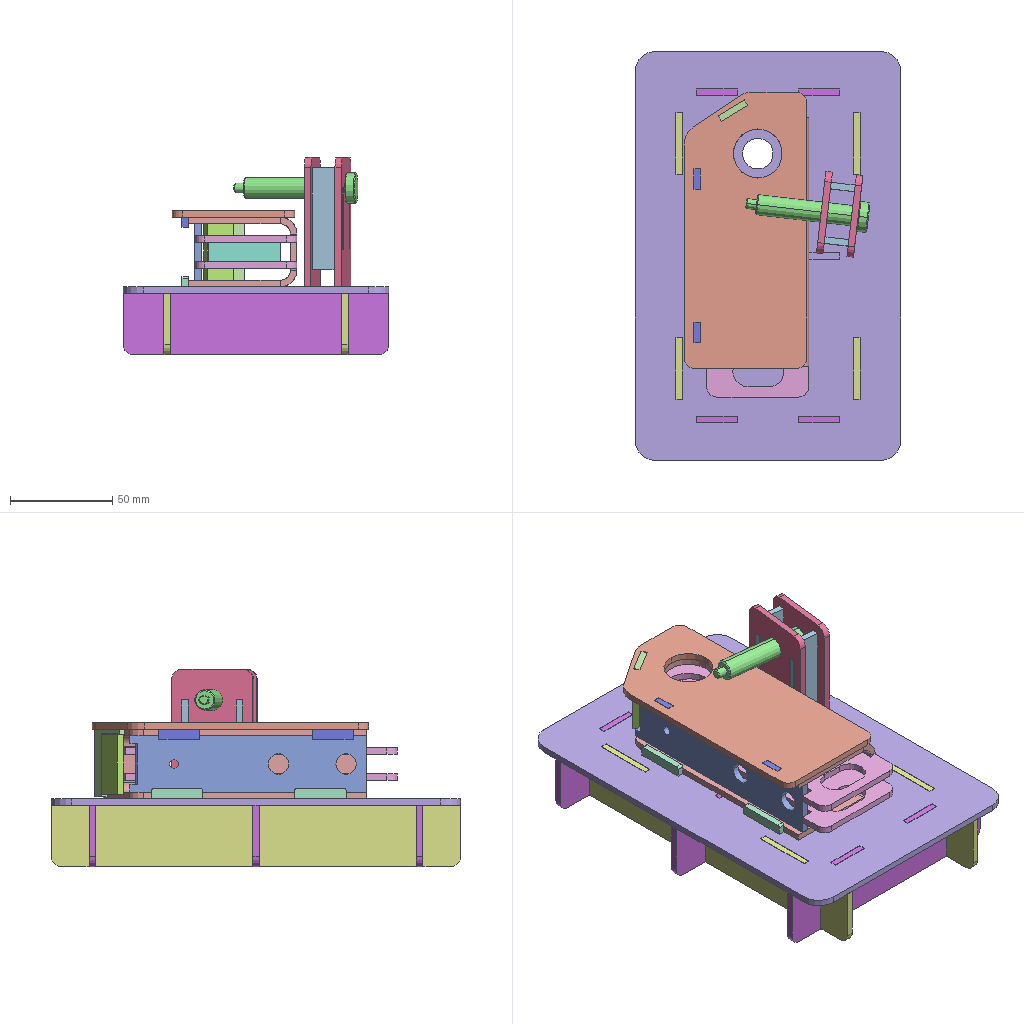Assembly | SolidWorks | 16 different items | 25 placed | box 130 x 200 x 97 mm
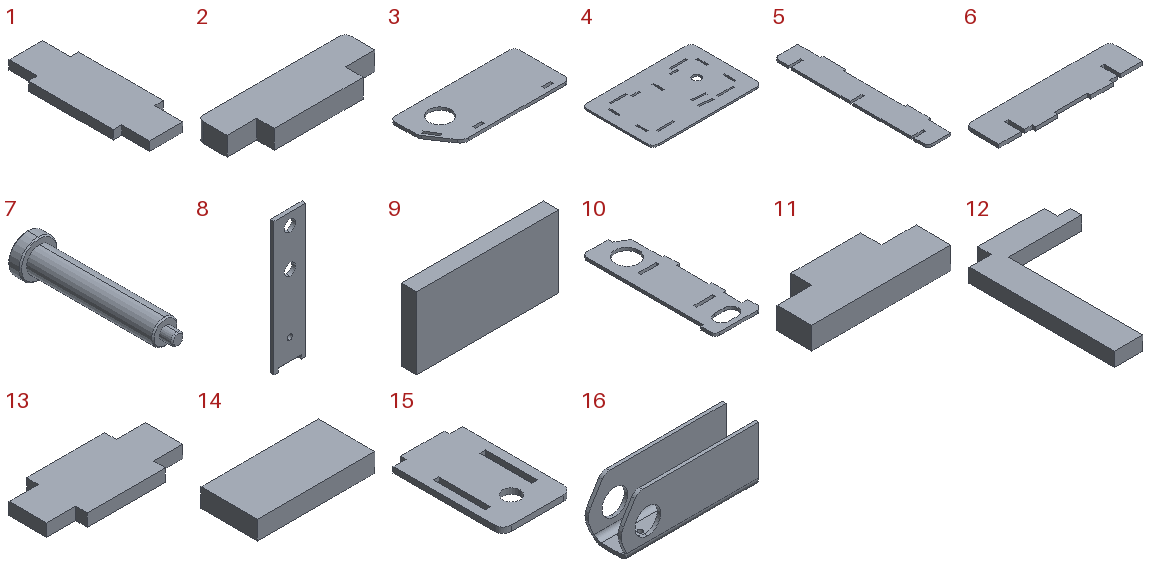Parts list (item | quantity | size | volume | features):
1 | x2 | 17.8 x 50 x 3.2 mm | 2464 mm3 | features FlatPattern 1, SMBaseFlange 1, SheetMetal 1
2 | x2 | 25 x 8 x 3.2 mm | 542.627 mm3 | features FlatPattern 1, SMBaseFlange 1, SheetMetal 1
3 | x1 | 135 x 60 x 3.2 mm | 23086 mm3 | features FlatPattern 1, SMBaseFlange 1, SheetMetal 1
4 | x1 | 200 x 130 x 3.2 mm | 79288 mm3 | features FlatPattern 1, SMBaseFlange 1, SheetMetal 1
5 | x2 | 33 x 200 x 3.2 mm | 19266 mm3 | features FlatPattern 1, SMBaseFlange 1, SheetMetal 1
6 | x3 | 130 x 33 x 3.2 mm | 12522 mm3 | features FlatPattern 1, SMBaseFlange 1, SheetMetal 1
7 | x1 | 15 x 60 x 15 mm | 4886 mm3 | features Chamfer 1, Revolution 1
8 | x1 | 27.6 x 3.2 x 115.6 mm | 9476 mm3 | features Chamfer 1, FlatPattern 1, SMBaseFlange 1, SheetMetal 1
9 | x1 | 29.6 x 3.2 x 15 mm | 1421 mm3 | features FlatPattern 1, SMBaseFlange 1, SheetMetal 1
10 | x2 | 50 x 145 x 3.2 mm | 16071 mm3 | features Fillet 1, FlatPattern 1, SMBaseFlange 1, SheetMetal 1
11 | x2 | 20 x 8 x 3.2 mm | 416 mm3 | features FlatPattern 1, SMBaseFlange 1, SheetMetal 1
12 | x1 | 23 x 36 x 3.2 mm | 953.226 mm3 | features FlatPattern 1, SMBaseFlange 1, SheetMetal 1
13 | x2 | 35 x 15.6 x 3.2 mm | 1459 mm3 | features FlatPattern 1, SMBaseFlange 1, SheetMetal 1
14 | x1 | 20 x 9.6 x 3.2 mm | 614.4 mm3 | features FlatPattern 1, SMBaseFlange 1, SheetMetal 1
15 | x2 | 40 x 66.3 x 3.2 mm | 7442 mm3 | features Fillet 1, FlatPattern 1, SMBaseFlange 1, SheetMetal 1
16 | x1 | 128.757 x 34 x 53 mm | 47449 mm3 | features ICE 2, Fillet 1, FlatPattern 1, SMBaseFlange 1, SheetMetal 1
Mates (type | each side: item.copy, entity, surface, feature):
Coincident | 16.1 face plane Base-Flange1 | 8.1 face plane Base-Flange1 | 2 times
DistanceDim | 16.1 face plane Base-Flange1 | 8.1 face plane Base-Flange1
Coincident | 16.1 face plane Cut-Extrude1 | 9.1 face plane Base-Flange1
DistanceDim | 9.1 face plane Base-Flange1 | 16.1 face plane Base-Flange1
DistanceDim | 9.1 edge | 16.1 face plane Base-Flange1
InPlace | 10.1 plane | assembly plane
InPlace | 13.1 plane | assembly plane
InPlace | 14.1 plane | assembly plane
Coincident | 16.1 face plane Base-Flange1 | 4.1 face plane Base-Flange1
Concentric | 16.1 face cylinder Cut-Extrude1 | 4.1 face cylinder Base-Flange1
Parallel | 16.1 face plane Base-Flange1 | 4.1 face plane Base-Flange1
InPlace | 7.1 face plane Revolve1 | 15.1 plane
InPlace | 1.1 plane | assembly plane
InPlace | 5.1 plane | assembly plane
InPlace | 6.1 plane | assembly plane
InPlace | 16.1 face plane Base-Flange1 | 2.1 plane
InPlace | 16.1 face plane Base-Flange1 | 3.1 plane
InPlace | 16.1 face plane Base-Flange1 | 11.1 plane
InPlace | 16.1 face plane Cut-Extrude1 | 12.1 plane